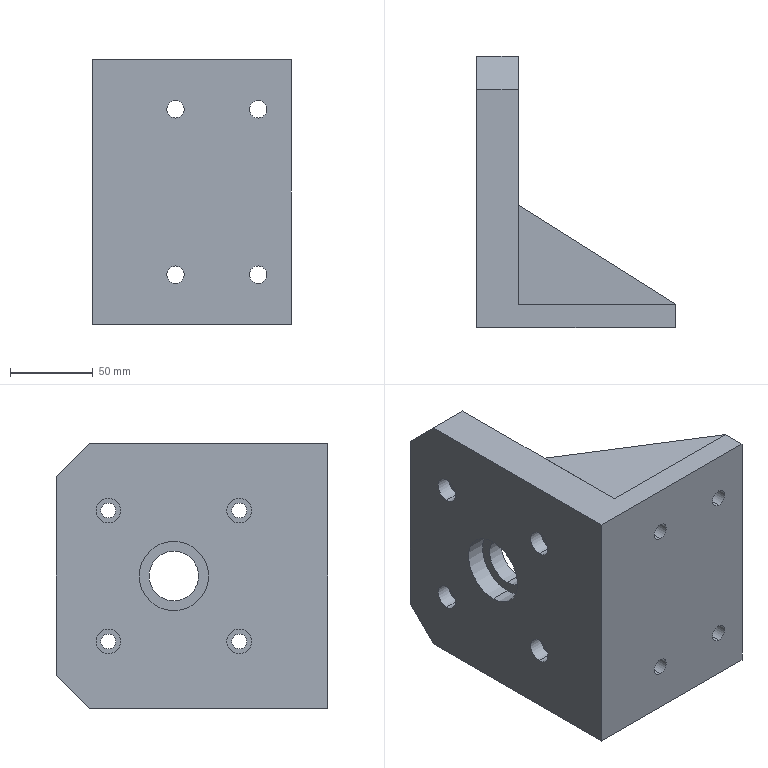Part | SolidWorks | features ICE 6, HoleWzd 2, Chamfer 1, CirPattern 1, Extrusion 1, LPattern 1 | 3 solids | 56 faces | box 120 x 164 x 160 mm | volume 840772 mm3 | cylinder 30 | plane 26 | commonest cylinder face diameters 9 x8 10.5 x8 15 x8 30 x2 42 x2 125 x2